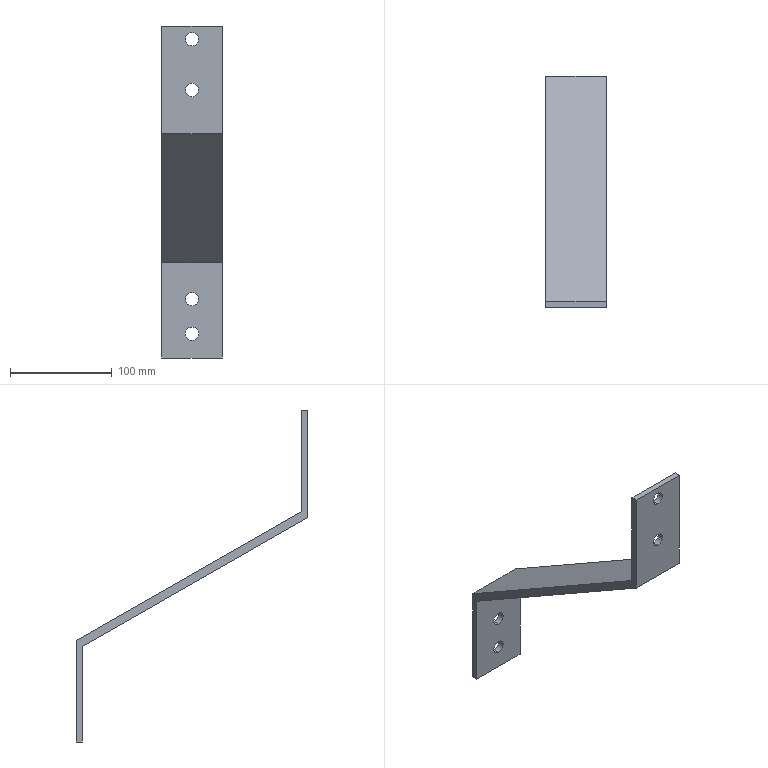Part | SolidWorks | features BaseBody 1 | 1 solid | 18 faces | box 60 x 228 x 327 mm | volume 194454 mm3 | plane 10 | cylinder 8 | commonest cylinder face diameters 13 x8
STEP:
#1=CARTESIAN_POINT('',(756.946,-3258.723,1045.471));
#2=VERTEX_POINT('',#1);
#3=CARTESIAN_POINT('',(756.946,-3258.723,1032.471));
#4=VERTEX_POINT('',#3);
#5=CARTESIAN_POINT('',(756.946,-3258.723,1038.971));
#6=DIRECTION('',(0.,-1.,0.));
#7=DIRECTION('',(0.,0.,-1.));
#8=AXIS2_PLACEMENT_3D('',#5,#6,#7);
#9=CIRCLE('',#8,6.5);
#10=EDGE_CURVE('',#2,#4,#9,.T.);
#11=ORIENTED_EDGE('',*,*,#10,.F.);
#12=CARTESIAN_POINT('',(756.946,-3264.723,1045.471));
#13=VERTEX_POINT('',#12);
#14=CARTESIAN_POINT('',(756.946,-3284.572,1045.471));
#15=DIRECTION('',(0.,-1.,0.));
#16=VECTOR('',#15,1000.);
#17=LINE('',#14,#16);
#18=EDGE_CURVE('',#2,#13,#17,.T.);
#19=ORIENTED_EDGE('',*,*,#18,.T.);
#20=CARTESIAN_POINT('',(756.946,-3264.723,1032.471));
#21=VERTEX_POINT('',#20);
#22=CARTESIAN_POINT('',(756.946,-3264.723,1038.971));
#23=DIRECTION('',(0.,1.,0.));
#24=DIRECTION('',(0.,0.,-1.));
#25=AXIS2_PLACEMENT_3D('',#22,#23,#24);
#26=CIRCLE('',#25,6.5);
#27=EDGE_CURVE('',#21,#13,#26,.T.);
#28=ORIENTED_EDGE('',*,*,#27,.F.);
#29=CARTESIAN_POINT('',(756.946,-3284.572,1032.471));
#30=DIRECTION('',(0.,-1.,0.));
#31=VECTOR('',#30,1000.);
#32=LINE('',#29,#31);
#33=EDGE_CURVE('',#4,#21,#32,.T.);
#34=ORIENTED_EDGE('',*,*,#33,.F.);
#35=EDGE_LOOP('',(#11,#19,#28,#34));
#36=FACE_OUTER_BOUND('',#35,.T.);
#37=CARTESIAN_POINT('',(756.946,-3284.572,1038.971));
#38=DIRECTION('',(0.,-1.,0.));
#39=DIRECTION('',(0.,0.,-1.));
#40=AXIS2_PLACEMENT_3D('',#37,#38,#39);
#41=CYLINDRICAL_SURFACE('',#40,6.5);
#42=ADVANCED_FACE('',(#36),#41,.F.);
#43=CARTESIAN_POINT('',(756.946,-3258.723,1079.471));
#44=VERTEX_POINT('',#43);
#45=CARTESIAN_POINT('',(756.946,-3258.723,1066.471));
#46=VERTEX_POINT('',#45);
#47=CARTESIAN_POINT('',(756.946,-3258.723,1072.971));
#48=DIRECTION('',(0.,-1.,0.));
#49=DIRECTION('',(0.,0.,-1.));
#50=AXIS2_PLACEMENT_3D('',#47,#48,#49);
#51=CIRCLE('',#50,6.5);
#52=EDGE_CURVE('',#44,#46,#51,.T.);
#53=ORIENTED_EDGE('',*,*,#52,.F.);
#54=CARTESIAN_POINT('',(756.946,-3264.723,1079.471));
#55=VERTEX_POINT('',#54);
#56=CARTESIAN_POINT('',(756.946,-3284.572,1079.471));
#57=DIRECTION('',(0.,-1.,0.));
#58=VECTOR('',#57,1000.);
#59=LINE('',#56,#58);
#60=EDGE_CURVE('',#44,#55,#59,.T.);
#61=ORIENTED_EDGE('',*,*,#60,.T.);
#62=CARTESIAN_POINT('',(756.946,-3264.723,1066.471));
#63=VERTEX_POINT('',#62);
#64=CARTESIAN_POINT('',(756.946,-3264.723,1072.971));
#65=DIRECTION('',(0.,1.,0.));
#66=DIRECTION('',(0.,0.,-1.));
#67=AXIS2_PLACEMENT_3D('',#64,#65,#66);
#68=CIRCLE('',#67,6.5);
#69=EDGE_CURVE('',#63,#55,#68,.T.);
#70=ORIENTED_EDGE('',*,*,#69,.F.);
#71=CARTESIAN_POINT('',(756.946,-3284.572,1066.471));
#72=DIRECTION('',(0.,-1.,0.));
#73=VECTOR('',#72,1000.);
#74=LINE('',#71,#73);
#75=EDGE_CURVE('',#46,#63,#74,.T.);
#76=ORIENTED_EDGE('',*,*,#75,.F.);
#77=EDGE_LOOP('',(#53,#61,#70,#76));
#78=FACE_OUTER_BOUND('',#77,.T.);
#79=CARTESIAN_POINT('',(756.946,-3284.572,1072.971));
#80=DIRECTION('',(0.,-1.,0.));
#81=DIRECTION('',(0.,0.,-1.));
#82=AXIS2_PLACEMENT_3D('',#79,#80,#81);
#83=CYLINDRICAL_SURFACE('',#82,6.5);
#84=ADVANCED_FACE('',(#78),#83,.F.);
#85=CARTESIAN_POINT('',(756.946,-3480.723,1335.471));
#86=VERTEX_POINT('',#85);
#87=CARTESIAN_POINT('',(756.946,-3480.723,1322.471));
#88=VERTEX_POINT('',#87);
#89=CARTESIAN_POINT('',(756.946,-3480.723,1328.971));
#90=DIRECTION('',(0.,-1.,0.));
#91=DIRECTION('',(0.,0.,-1.));
#92=AXIS2_PLACEMENT_3D('',#89,#90,#91);
#93=CIRCLE('',#92,6.5);
#94=EDGE_CURVE('',#86,#88,#93,.T.);
#95=ORIENTED_EDGE('',*,*,#94,.F.);
#96=CARTESIAN_POINT('',(756.946,-3486.723,1335.471));
#97=VERTEX_POINT('',#96);
#98=CARTESIAN_POINT('',(756.946,-3470.551,1335.471));
#99=DIRECTION('',(0.,-1.,0.));
#100=VECTOR('',#99,1000.);
#101=LINE('',#98,#100);
#102=EDGE_CURVE('',#86,#97,#101,.T.);
#103=ORIENTED_EDGE('',*,*,#102,.T.);
#104=CARTESIAN_POINT('',(756.946,-3486.723,1322.471));
#105=VERTEX_POINT('',#104);
#106=CARTESIAN_POINT('',(756.946,-3486.723,1328.971));
#107=DIRECTION('',(0.,1.,0.));
#108=DIRECTION('',(0.,0.,-1.));
#109=AXIS2_PLACEMENT_3D('',#106,#107,#108);
#110=CIRCLE('',#109,6.5);
#111=EDGE_CURVE('',#105,#97,#110,.T.);
#112=ORIENTED_EDGE('',*,*,#111,.F.);
#113=CARTESIAN_POINT('',(756.946,-3470.551,1322.471));
#114=DIRECTION('',(0.,-1.,0.));
#115=VECTOR('',#114,1000.);
#116=LINE('',#113,#115);
#117=EDGE_CURVE('',#88,#105,#116,.T.);
#118=ORIENTED_EDGE('',*,*,#117,.F.);
#119=EDGE_LOOP('',(#95,#103,#112,#118));
#120=FACE_OUTER_BOUND('',#119,.T.);
#121=CARTESIAN_POINT('',(756.946,-3470.551,1328.971));
#122=DIRECTION('',(0.,-1.,0.));
#123=DIRECTION('',(0.,0.,-1.));
#124=AXIS2_PLACEMENT_3D('',#121,#122,#123);
#125=CYLINDRICAL_SURFACE('',#124,6.5);
#126=ADVANCED_FACE('',(#120),#125,.F.);
#127=CARTESIAN_POINT('',(756.946,-3480.723,1285.471));
#128=VERTEX_POINT('',#127);
#129=CARTESIAN_POINT('',(756.946,-3480.723,1272.471));
#130=VERTEX_POINT('',#129);
#131=CARTESIAN_POINT('',(756.946,-3480.723,1278.971));
#132=DIRECTION('',(0.,-1.,0.));
#133=DIRECTION('',(0.,0.,-1.));
#134=AXIS2_PLACEMENT_3D('',#131,#132,#133);
#135=CIRCLE('',#134,6.5);
#136=EDGE_CURVE('',#128,#130,#135,.T.);
#137=ORIENTED_EDGE('',*,*,#136,.F.);
#138=CARTESIAN_POINT('',(756.946,-3486.723,1285.471));
#139=VERTEX_POINT('',#138);
#140=CARTESIAN_POINT('',(756.946,-3470.551,1285.471));
#141=DIRECTION('',(0.,-1.,0.));
#142=VECTOR('',#141,1000.);
#143=LINE('',#140,#142);
#144=EDGE_CURVE('',#128,#139,#143,.T.);
#145=ORIENTED_EDGE('',*,*,#144,.T.);
#146=CARTESIAN_POINT('',(756.946,-3486.723,1272.471));
#147=VERTEX_POINT('',#146);
#148=CARTESIAN_POINT('',(756.946,-3486.723,1278.971));
#149=DIRECTION('',(0.,1.,0.));
#150=DIRECTION('',(0.,0.,-1.));
#151=AXIS2_PLACEMENT_3D('',#148,#149,#150);
#152=CIRCLE('',#151,6.5);
#153=EDGE_CURVE('',#147,#139,#152,.T.);
#154=ORIENTED_EDGE('',*,*,#153,.F.);
#155=CARTESIAN_POINT('',(756.946,-3470.551,1272.471));
#156=DIRECTION('',(0.,-1.,0.));
#157=VECTOR('',#156,1000.);
#158=LINE('',#155,#157);
#159=EDGE_CURVE('',#130,#147,#158,.T.);
#160=ORIENTED_EDGE('',*,*,#159,.F.);
#161=EDGE_LOOP('',(#137,#145,#154,#160));
#162=FACE_OUTER_BOUND('',#161,.T.);
#163=CARTESIAN_POINT('',(756.946,-3470.551,1278.971));
#164=DIRECTION('',(0.,-1.,0.));
#165=DIRECTION('',(0.,0.,-1.));
#166=AXIS2_PLACEMENT_3D('',#163,#164,#165);
#167=CYLINDRICAL_SURFACE('',#166,6.5);
#168=ADVANCED_FACE('',(#162),#167,.F.);
#169=CARTESIAN_POINT('',(786.946,-3480.723,1241.971));
#170=VERTEX_POINT('',#169);
#171=CARTESIAN_POINT('',(786.946,-3258.723,1114.971));
#172=VERTEX_POINT('',#171);
#173=CARTESIAN_POINT('',(786.946,-3258.723,1114.971));
#174=DIRECTION('',(0.,0.868,-0.4966));
#175=VECTOR('',#174,1000.);
#176=LINE('',#173,#175);
#177=EDGE_CURVE('',#170,#172,#176,.T.);
#178=ORIENTED_EDGE('',*,*,#177,.T.);
#179=CARTESIAN_POINT('',(726.946,-3258.723,1114.971));
#180=VERTEX_POINT('',#179);
#181=CARTESIAN_POINT('',(786.946,-3258.723,1114.971));
#182=DIRECTION('',(-1.,0.,0.));
#183=VECTOR('',#182,1000.);
#184=LINE('',#181,#183);
#185=EDGE_CURVE('',#172,#180,#184,.T.);
#186=ORIENTED_EDGE('',*,*,#185,.T.);
#187=CARTESIAN_POINT('',(726.946,-3480.723,1241.971));
#188=VERTEX_POINT('',#187);
#189=CARTESIAN_POINT('',(726.946,-3258.723,1114.971));
#190=DIRECTION('',(0.,-0.868,0.4966));
#191=VECTOR('',#190,1000.);
#192=LINE('',#189,#191);
#193=EDGE_CURVE('',#180,#188,#192,.T.);
#194=ORIENTED_EDGE('',*,*,#193,.T.);
#195=CARTESIAN_POINT('',(786.946,-3480.723,1241.971));
#196=DIRECTION('',(1.,0.,0.));
#197=VECTOR('',#196,1000.);
#198=LINE('',#195,#197);
#199=EDGE_CURVE('',#188,#170,#198,.T.);
#200=ORIENTED_EDGE('',*,*,#199,.T.);
#201=EDGE_LOOP('',(#178,#186,#194,#200));
#202=FACE_OUTER_BOUND('',#201,.T.);
#203=CARTESIAN_POINT('',(786.946,-3258.723,1114.971));
#204=DIRECTION('',(0.,0.4966,0.868));
#205=DIRECTION('',(0.,-0.868,0.4966));
#206=AXIS2_PLACEMENT_3D('',#203,#204,#205);
#207=PLANE('',#206);
#208=ADVANCED_FACE('',(#202),#207,.T.);
#209=CARTESIAN_POINT('',(786.946,-3258.723,1014.971));
#210=VERTEX_POINT('',#209);
#211=CARTESIAN_POINT('',(786.946,-3258.723,1014.971));
#212=DIRECTION('',(0.,0.,-1.));
#213=VECTOR('',#212,1000.);
#214=LINE('',#211,#213);
#215=EDGE_CURVE('',#172,#210,#214,.T.);
#216=ORIENTED_EDGE('',*,*,#215,.T.);
#217=CARTESIAN_POINT('',(726.946,-3258.723,1014.971));
#218=VERTEX_POINT('',#217);
#219=CARTESIAN_POINT('',(786.946,-3258.723,1014.971));
#220=DIRECTION('',(-1.,0.,0.));
#221=VECTOR('',#220,1000.);
#222=LINE('',#219,#221);
#223=EDGE_CURVE('',#210,#218,#222,.T.);
#224=ORIENTED_EDGE('',*,*,#223,.T.);
#225=CARTESIAN_POINT('',(726.946,-3258.723,1014.971));
#226=DIRECTION('',(0.,0.,1.));
#227=VECTOR('',#226,1000.);
#228=LINE('',#225,#227);
#229=EDGE_CURVE('',#218,#180,#228,.T.);
#230=ORIENTED_EDGE('',*,*,#229,.T.);
#231=ORIENTED_EDGE('',*,*,#185,.F.);
#232=EDGE_LOOP('',(#216,#224,#230,#231));
#233=FACE_OUTER_BOUND('',#232,.T.);
#234=CARTESIAN_POINT('',(756.946,-3258.723,1038.971));
#235=DIRECTION('',(0.,-1.,0.));
#236=DIRECTION('',(0.,0.,-1.));
#237=AXIS2_PLACEMENT_3D('',#234,#235,#236);
#238=CIRCLE('',#237,6.5);
#239=EDGE_CURVE('',#4,#2,#238,.T.);
#240=ORIENTED_EDGE('',*,*,#239,.T.);
#241=ORIENTED_EDGE('',*,*,#10,.T.);
#242=EDGE_LOOP('',(#240,#241));
#243=FACE_BOUND('',#242,.T.);
#244=CARTESIAN_POINT('',(756.946,-3258.723,1072.971));
#245=DIRECTION('',(0.,-1.,0.));
#246=DIRECTION('',(0.,0.,-1.));
#247=AXIS2_PLACEMENT_3D('',#244,#245,#246);
#248=CIRCLE('',#247,6.5);
#249=EDGE_CURVE('',#46,#44,#248,.T.);
#250=ORIENTED_EDGE('',*,*,#249,.T.);
#251=ORIENTED_EDGE('',*,*,#52,.T.);
#252=EDGE_LOOP('',(#250,#251));
#253=FACE_BOUND('',#252,.T.);
#254=CARTESIAN_POINT('',(786.946,-3258.723,1014.971));
#255=DIRECTION('',(0.,1.,0.));
#256=DIRECTION('',(0.,0.,1.));
#257=AXIS2_PLACEMENT_3D('',#254,#255,#256);
#258=PLANE('',#257);
#259=ADVANCED_FACE('',(#233,#243,#253),#258,.T.);
#260=CARTESIAN_POINT('',(786.946,-3264.723,1108.971));
#261=VERTEX_POINT('',#260);
#262=CARTESIAN_POINT('',(786.946,-3264.723,1014.971));
#263=VERTEX_POINT('',#262);
#264=CARTESIAN_POINT('',(786.946,-3264.723,1177.635));
#265=DIRECTION('',(0.,0.,-1.));
#266=VECTOR('',#265,1000.);
#267=LINE('',#264,#266);
#268=EDGE_CURVE('',#261,#263,#267,.T.);
#269=ORIENTED_EDGE('',*,*,#268,.T.);
#270=CARTESIAN_POINT('',(786.946,-3374.165,1014.971));
#271=DIRECTION('',(0.,1.,0.));
#272=VECTOR('',#271,1000.);
#273=LINE('',#270,#272);
#274=EDGE_CURVE('',#263,#210,#273,.T.);
#275=ORIENTED_EDGE('',*,*,#274,.T.);
#276=ORIENTED_EDGE('',*,*,#215,.F.);
#277=ORIENTED_EDGE('',*,*,#177,.F.);
#278=CARTESIAN_POINT('',(786.946,-3480.723,1341.971));
#279=VERTEX_POINT('',#278);
#280=CARTESIAN_POINT('',(786.946,-3480.723,1177.635));
#281=DIRECTION('',(0.,0.,1.));
#282=VECTOR('',#281,1000.);
#283=LINE('',#280,#282);
#284=EDGE_CURVE('',#170,#279,#283,.T.);
#285=ORIENTED_EDGE('',*,*,#284,.T.);
#286=CARTESIAN_POINT('',(786.946,-3486.723,1341.971));
#287=VERTEX_POINT('',#286);
#288=CARTESIAN_POINT('',(786.946,-3374.165,1341.971));
#289=DIRECTION('',(0.,-1.,0.));
#290=VECTOR('',#289,1000.);
#291=LINE('',#288,#290);
#292=EDGE_CURVE('',#279,#287,#291,.T.);
#293=ORIENTED_EDGE('',*,*,#292,.T.);
#294=CARTESIAN_POINT('',(786.946,-3486.723,1235.971));
#295=VERTEX_POINT('',#294);
#296=CARTESIAN_POINT('',(786.946,-3486.723,1177.635));
#297=DIRECTION('',(0.,0.,-1.));
#298=VECTOR('',#297,1000.);
#299=LINE('',#296,#298);
#300=EDGE_CURVE('',#287,#295,#299,.T.);
#301=ORIENTED_EDGE('',*,*,#300,.T.);
#302=CARTESIAN_POINT('',(786.946,-3486.723,1235.971));
#303=DIRECTION('',(0.,0.868,-0.4966));
#304=VECTOR('',#303,1000.);
#305=LINE('',#302,#304);
#306=EDGE_CURVE('',#295,#261,#305,.T.);
#307=ORIENTED_EDGE('',*,*,#306,.T.);
#308=EDGE_LOOP('',(#269,#275,#276,#277,#285,#293,#301,#307));
#309=FACE_OUTER_BOUND('',#308,.T.);
#310=CARTESIAN_POINT('',(786.946,-3374.165,1177.635));
#311=DIRECTION('',(1.,0.,0.));
#312=DIRECTION('',(0.,1.,0.));
#313=AXIS2_PLACEMENT_3D('',#310,#311,#312);
#314=PLANE('',#313);
#315=ADVANCED_FACE('',(#309),#314,.T.);
#316=ORIENTED_EDGE('',*,*,#284,.F.);
#317=ORIENTED_EDGE('',*,*,#199,.F.);
#318=CARTESIAN_POINT('',(726.946,-3480.723,1341.971));
#319=VERTEX_POINT('',#318);
#320=CARTESIAN_POINT('',(726.946,-3480.723,1241.971));
#321=DIRECTION('',(0.,0.,1.));
#322=VECTOR('',#321,1000.);
#323=LINE('',#320,#322);
#324=EDGE_CURVE('',#188,#319,#323,.T.);
#325=ORIENTED_EDGE('',*,*,#324,.T.);
#326=CARTESIAN_POINT('',(786.946,-3480.723,1341.971));
#327=DIRECTION('',(1.,0.,0.));
#328=VECTOR('',#327,1000.);
#329=LINE('',#326,#328);
#330=EDGE_CURVE('',#319,#279,#329,.T.);
#331=ORIENTED_EDGE('',*,*,#330,.T.);
#332=EDGE_LOOP('',(#316,#317,#325,#331));
#333=FACE_OUTER_BOUND('',#332,.T.);
#334=CARTESIAN_POINT('',(756.946,-3480.723,1328.971));
#335=DIRECTION('',(0.,-1.,0.));
#336=DIRECTION('',(0.,0.,-1.));
#337=AXIS2_PLACEMENT_3D('',#334,#335,#336);
#338=CIRCLE('',#337,6.5);
#339=EDGE_CURVE('',#88,#86,#338,.T.);
#340=ORIENTED_EDGE('',*,*,#339,.T.);
#341=ORIENTED_EDGE('',*,*,#94,.T.);
#342=EDGE_LOOP('',(#340,#341));
#343=FACE_BOUND('',#342,.T.);
#344=CARTESIAN_POINT('',(756.946,-3480.723,1278.971));
#345=DIRECTION('',(0.,-1.,0.));
#346=DIRECTION('',(0.,0.,-1.));
#347=AXIS2_PLACEMENT_3D('',#344,#345,#346);
#348=CIRCLE('',#347,6.5);
#349=EDGE_CURVE('',#130,#128,#348,.T.);
#350=ORIENTED_EDGE('',*,*,#349,.T.);
#351=ORIENTED_EDGE('',*,*,#136,.T.);
#352=EDGE_LOOP('',(#350,#351));
#353=FACE_BOUND('',#352,.T.);
#354=CARTESIAN_POINT('',(786.946,-3480.723,1241.971));
#355=DIRECTION('',(0.,1.,0.));
#356=DIRECTION('',(0.,0.,1.));
#357=AXIS2_PLACEMENT_3D('',#354,#355,#356);
#358=PLANE('',#357);
#359=ADVANCED_FACE('',(#333,#343,#353),#358,.T.);
#360=ORIENTED_EDGE('',*,*,#229,.F.);
#361=CARTESIAN_POINT('',(726.946,-3264.723,1014.971));
#362=VERTEX_POINT('',#361);
#363=CARTESIAN_POINT('',(726.946,-3374.165,1014.971));
#364=DIRECTION('',(0.,1.,0.));
#365=VECTOR('',#364,1000.);
#366=LINE('',#363,#365);
#367=EDGE_CURVE('',#362,#218,#366,.T.);
#368=ORIENTED_EDGE('',*,*,#367,.F.);
#369=CARTESIAN_POINT('',(726.946,-3264.723,1108.971));
#370=VERTEX_POINT('',#369);
#371=CARTESIAN_POINT('',(726.946,-3264.723,1177.635));
#372=DIRECTION('',(0.,0.,-1.));
#373=VECTOR('',#372,1000.);
#374=LINE('',#371,#373);
#375=EDGE_CURVE('',#370,#362,#374,.T.);
#376=ORIENTED_EDGE('',*,*,#375,.F.);
#377=CARTESIAN_POINT('',(726.946,-3486.723,1235.971));
#378=VERTEX_POINT('',#377);
#379=CARTESIAN_POINT('',(726.946,-3486.723,1235.971));
#380=DIRECTION('',(0.,0.868,-0.4966));
#381=VECTOR('',#380,1000.);
#382=LINE('',#379,#381);
#383=EDGE_CURVE('',#378,#370,#382,.T.);
#384=ORIENTED_EDGE('',*,*,#383,.F.);
#385=CARTESIAN_POINT('',(726.946,-3486.723,1341.971));
#386=VERTEX_POINT('',#385);
#387=CARTESIAN_POINT('',(726.946,-3486.723,1177.635));
#388=DIRECTION('',(0.,0.,-1.));
#389=VECTOR('',#388,1000.);
#390=LINE('',#387,#389);
#391=EDGE_CURVE('',#386,#378,#390,.T.);
#392=ORIENTED_EDGE('',*,*,#391,.F.);
#393=CARTESIAN_POINT('',(726.946,-3374.165,1341.971));
#394=DIRECTION('',(0.,-1.,0.));
#395=VECTOR('',#394,1000.);
#396=LINE('',#393,#395);
#397=EDGE_CURVE('',#319,#386,#396,.T.);
#398=ORIENTED_EDGE('',*,*,#397,.F.);
#399=ORIENTED_EDGE('',*,*,#324,.F.);
#400=ORIENTED_EDGE('',*,*,#193,.F.);
#401=EDGE_LOOP('',(#360,#368,#376,#384,#392,#398,#399,#400));
#402=FACE_OUTER_BOUND('',#401,.T.);
#403=CARTESIAN_POINT('',(726.946,-3374.165,1177.635));
#404=DIRECTION('',(1.,0.,0.));
#405=DIRECTION('',(0.,1.,0.));
#406=AXIS2_PLACEMENT_3D('',#403,#404,#405);
#407=PLANE('',#406);
#408=ADVANCED_FACE('',(#402),#407,.F.);
#409=ORIENTED_EDGE('',*,*,#274,.F.);
#410=CARTESIAN_POINT('',(786.946,-3264.723,1014.971));
#411=DIRECTION('',(-1.,0.,0.));
#412=VECTOR('',#411,1000.);
#413=LINE('',#410,#412);
#414=EDGE_CURVE('',#263,#362,#413,.T.);
#415=ORIENTED_EDGE('',*,*,#414,.T.);
#416=ORIENTED_EDGE('',*,*,#367,.T.);
#417=ORIENTED_EDGE('',*,*,#223,.F.);
#418=EDGE_LOOP('',(#409,#415,#416,#417));
#419=FACE_OUTER_BOUND('',#418,.T.);
#420=CARTESIAN_POINT('',(786.946,-3264.723,1014.971));
#421=DIRECTION('',(0.,0.,-1.));
#422=DIRECTION('',(-1.,0.,0.));
#423=AXIS2_PLACEMENT_3D('',#420,#421,#422);
#424=PLANE('',#423);
#425=ADVANCED_FACE('',(#419),#424,.T.);
#426=ORIENTED_EDGE('',*,*,#18,.F.);
#427=ORIENTED_EDGE('',*,*,#239,.F.);
#428=ORIENTED_EDGE('',*,*,#33,.T.);
#429=CARTESIAN_POINT('',(756.946,-3264.723,1038.971));
#430=DIRECTION('',(0.,1.,0.));
#431=DIRECTION('',(0.,0.,-1.));
#432=AXIS2_PLACEMENT_3D('',#429,#430,#431);
#433=CIRCLE('',#432,6.5);
#434=EDGE_CURVE('',#13,#21,#433,.T.);
#435=ORIENTED_EDGE('',*,*,#434,.F.);
#436=EDGE_LOOP('',(#426,#427,#428,#435));
#437=FACE_OUTER_BOUND('',#436,.T.);
#438=CARTESIAN_POINT('',(756.946,-3284.572,1038.971));
#439=DIRECTION('',(0.,-1.,0.));
#440=DIRECTION('',(0.,0.,-1.));
#441=AXIS2_PLACEMENT_3D('',#438,#439,#440);
#442=CYLINDRICAL_SURFACE('',#441,6.5);
#443=ADVANCED_FACE('',(#437),#442,.F.);
#444=ORIENTED_EDGE('',*,*,#60,.F.);
#445=ORIENTED_EDGE('',*,*,#249,.F.);
#446=ORIENTED_EDGE('',*,*,#75,.T.);
#447=CARTESIAN_POINT('',(756.946,-3264.723,1072.971));
#448=DIRECTION('',(0.,1.,0.));
#449=DIRECTION('',(0.,0.,-1.));
#450=AXIS2_PLACEMENT_3D('',#447,#448,#449);
#451=CIRCLE('',#450,6.5);
#452=EDGE_CURVE('',#55,#63,#451,.T.);
#453=ORIENTED_EDGE('',*,*,#452,.F.);
#454=EDGE_LOOP('',(#444,#445,#446,#453));
#455=FACE_OUTER_BOUND('',#454,.T.);
#456=CARTESIAN_POINT('',(756.946,-3284.572,1072.971));
#457=DIRECTION('',(0.,-1.,0.));
#458=DIRECTION('',(0.,0.,-1.));
#459=AXIS2_PLACEMENT_3D('',#456,#457,#458);
#460=CYLINDRICAL_SURFACE('',#459,6.5);
#461=ADVANCED_FACE('',(#455),#460,.F.);
#462=ORIENTED_EDGE('',*,*,#268,.F.);
#463=CARTESIAN_POINT('',(786.946,-3264.723,1108.971));
#464=DIRECTION('',(-1.,0.,0.));
#465=VECTOR('',#464,1000.);
#466=LINE('',#463,#465);
#467=EDGE_CURVE('',#261,#370,#466,.T.);
#468=ORIENTED_EDGE('',*,*,#467,.T.);
#469=ORIENTED_EDGE('',*,*,#375,.T.);
#470=ORIENTED_EDGE('',*,*,#414,.F.);
#471=EDGE_LOOP('',(#462,#468,#469,#470));
#472=FACE_OUTER_BOUND('',#471,.T.);
#473=ORIENTED_EDGE('',*,*,#27,.T.);
#474=ORIENTED_EDGE('',*,*,#434,.T.);
#475=EDGE_LOOP('',(#473,#474));
#476=FACE_BOUND('',#475,.T.);
#477=ORIENTED_EDGE('',*,*,#69,.T.);
#478=ORIENTED_EDGE('',*,*,#452,.T.);
#479=EDGE_LOOP('',(#477,#478));
#480=FACE_BOUND('',#479,.T.);
#481=CARTESIAN_POINT('',(786.946,-3264.723,1108.971));
#482=DIRECTION('',(0.,-1.,0.));
#483=DIRECTION('',(0.,0.,-1.));
#484=AXIS2_PLACEMENT_3D('',#481,#482,#483);
#485=PLANE('',#484);
#486=ADVANCED_FACE('',(#472,#476,#480),#485,.T.);
#487=ORIENTED_EDGE('',*,*,#306,.F.);
#488=CARTESIAN_POINT('',(786.946,-3486.723,1235.971));
#489=DIRECTION('',(-1.,0.,0.));
#490=VECTOR('',#489,1000.);
#491=LINE('',#488,#490);
#492=EDGE_CURVE('',#295,#378,#491,.T.);
#493=ORIENTED_EDGE('',*,*,#492,.T.);
#494=ORIENTED_EDGE('',*,*,#383,.T.);
#495=ORIENTED_EDGE('',*,*,#467,.F.);
#496=EDGE_LOOP('',(#487,#493,#494,#495));
#497=FACE_OUTER_BOUND('',#496,.T.);
#498=CARTESIAN_POINT('',(786.946,-3486.723,1235.971));
#499=DIRECTION('',(0.,-0.4966,-0.868));
#500=DIRECTION('',(0.,0.868,-0.4966));
#501=AXIS2_PLACEMENT_3D('',#498,#499,#500);
#502=PLANE('',#501);
#503=ADVANCED_FACE('',(#497),#502,.T.);
#504=ORIENTED_EDGE('',*,*,#300,.F.);
#505=CARTESIAN_POINT('',(786.946,-3486.723,1341.971));
#506=DIRECTION('',(-1.,0.,0.));
#507=VECTOR('',#506,1000.);
#508=LINE('',#505,#507);
#509=EDGE_CURVE('',#287,#386,#508,.T.);
#510=ORIENTED_EDGE('',*,*,#509,.T.);
#511=ORIENTED_EDGE('',*,*,#391,.T.);
#512=ORIENTED_EDGE('',*,*,#492,.F.);
#513=EDGE_LOOP('',(#504,#510,#511,#512));
#514=FACE_OUTER_BOUND('',#513,.T.);
#515=ORIENTED_EDGE('',*,*,#111,.T.);
#516=CARTESIAN_POINT('',(756.946,-3486.723,1328.971));
#517=DIRECTION('',(0.,1.,0.));
#518=DIRECTION('',(0.,0.,-1.));
#519=AXIS2_PLACEMENT_3D('',#516,#517,#518);
#520=CIRCLE('',#519,6.5);
#521=EDGE_CURVE('',#97,#105,#520,.T.);
#522=ORIENTED_EDGE('',*,*,#521,.T.);
#523=EDGE_LOOP('',(#515,#522));
#524=FACE_BOUND('',#523,.T.);
#525=ORIENTED_EDGE('',*,*,#153,.T.);
#526=CARTESIAN_POINT('',(756.946,-3486.723,1278.971));
#527=DIRECTION('',(0.,1.,0.));
#528=DIRECTION('',(0.,0.,-1.));
#529=AXIS2_PLACEMENT_3D('',#526,#527,#528);
#530=CIRCLE('',#529,6.5);
#531=EDGE_CURVE('',#139,#147,#530,.T.);
#532=ORIENTED_EDGE('',*,*,#531,.T.);
#533=EDGE_LOOP('',(#525,#532));
#534=FACE_BOUND('',#533,.T.);
#535=CARTESIAN_POINT('',(786.946,-3486.723,1341.971));
#536=DIRECTION('',(0.,-1.,0.));
#537=DIRECTION('',(0.,0.,-1.));
#538=AXIS2_PLACEMENT_3D('',#535,#536,#537);
#539=PLANE('',#538);
#540=ADVANCED_FACE('',(#514,#524,#534),#539,.T.);
#541=ORIENTED_EDGE('',*,*,#292,.F.);
#542=ORIENTED_EDGE('',*,*,#330,.F.);
#543=ORIENTED_EDGE('',*,*,#397,.T.);
#544=ORIENTED_EDGE('',*,*,#509,.F.);
#545=EDGE_LOOP('',(#541,#542,#543,#544));
#546=FACE_OUTER_BOUND('',#545,.T.);
#547=CARTESIAN_POINT('',(786.946,-3480.723,1341.971));
#548=DIRECTION('',(0.,0.,1.));
#549=DIRECTION('',(1.,0.,0.));
#550=AXIS2_PLACEMENT_3D('',#547,#548,#549);
#551=PLANE('',#550);
#552=ADVANCED_FACE('',(#546),#551,.T.);
#553=ORIENTED_EDGE('',*,*,#102,.F.);
#554=ORIENTED_EDGE('',*,*,#339,.F.);
#555=ORIENTED_EDGE('',*,*,#117,.T.);
#556=ORIENTED_EDGE('',*,*,#521,.F.);
#557=EDGE_LOOP('',(#553,#554,#555,#556));
#558=FACE_OUTER_BOUND('',#557,.T.);
#559=CARTESIAN_POINT('',(756.946,-3470.551,1328.971));
#560=DIRECTION('',(0.,-1.,0.));
#561=DIRECTION('',(0.,0.,-1.));
#562=AXIS2_PLACEMENT_3D('',#559,#560,#561);
#563=CYLINDRICAL_SURFACE('',#562,6.5);
#564=ADVANCED_FACE('',(#558),#563,.F.);
#565=ORIENTED_EDGE('',*,*,#144,.F.);
#566=ORIENTED_EDGE('',*,*,#349,.F.);
#567=ORIENTED_EDGE('',*,*,#159,.T.);
#568=ORIENTED_EDGE('',*,*,#531,.F.);
#569=EDGE_LOOP('',(#565,#566,#567,#568));
#570=FACE_OUTER_BOUND('',#569,.T.);
#571=CARTESIAN_POINT('',(756.946,-3470.551,1278.971));
#572=DIRECTION('',(0.,-1.,0.));
#573=DIRECTION('',(0.,0.,-1.));
#574=AXIS2_PLACEMENT_3D('',#571,#572,#573);
#575=CYLINDRICAL_SURFACE('',#574,6.5);
#576=ADVANCED_FACE('',(#570),#575,.F.);
#577=CLOSED_SHELL('',(#42,#84,#126,#168,#208,#259,#315,#359,#408,#425,#443,#461,#486,#503,#540,#552,#564,#576));
#578=MANIFOLD_SOLID_BREP('',#577);
#579=CARTESIAN_POINT('',(0.,0.,0.));
#580=DIRECTION('',(0.,0.,1.));
#581=DIRECTION('',(1.,0.,0.));
#582=AXIS2_PLACEMENT_3D('',#579,#580,#581);
#583=(LENGTH_UNIT()NAMED_UNIT(*)SI_UNIT(.MILLI.,.METRE.));
#584=UNCERTAINTY_MEASURE_WITH_UNIT(LENGTH_MEASURE(0.00001),#583,'','');
#585=(NAMED_UNIT(*)PLANE_ANGLE_UNIT()SI_UNIT($,.RADIAN.));
#586=(NAMED_UNIT(*)SI_UNIT($,.STERADIAN.)SOLID_ANGLE_UNIT());
#587=(GEOMETRIC_REPRESENTATION_CONTEXT(3)GLOBAL_UNCERTAINTY_ASSIGNED_CONTEXT((#584))GLOBAL_UNIT_ASSIGNED_CONTEXT((#583,#585,#586))REPRESENTATION_CONTEXT('',''));
#588=ADVANCED_BREP_SHAPE_REPRESENTATION('',(#578,#582),#587);